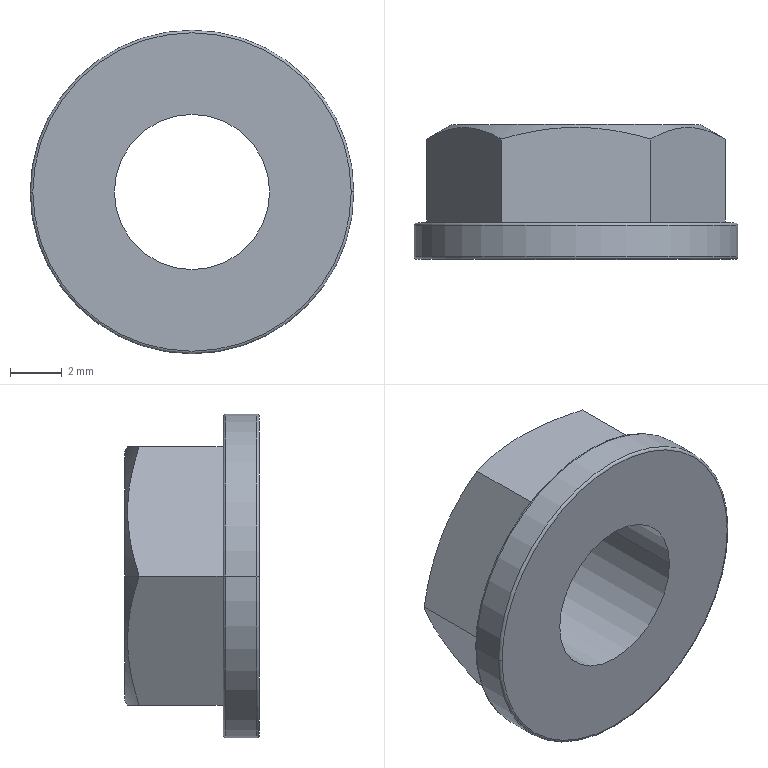Part | STEP file | LIB_68452317_M6_SERPRESS | 1 solid | 19 faces | box 12.5 x 5.2 x 12.5 mm | volume 351.327 mm3 | plane 9 | cylinder 4 | torus 4 | cone 2 | commonest cylinder face diameters 6 x2 12.5 x2